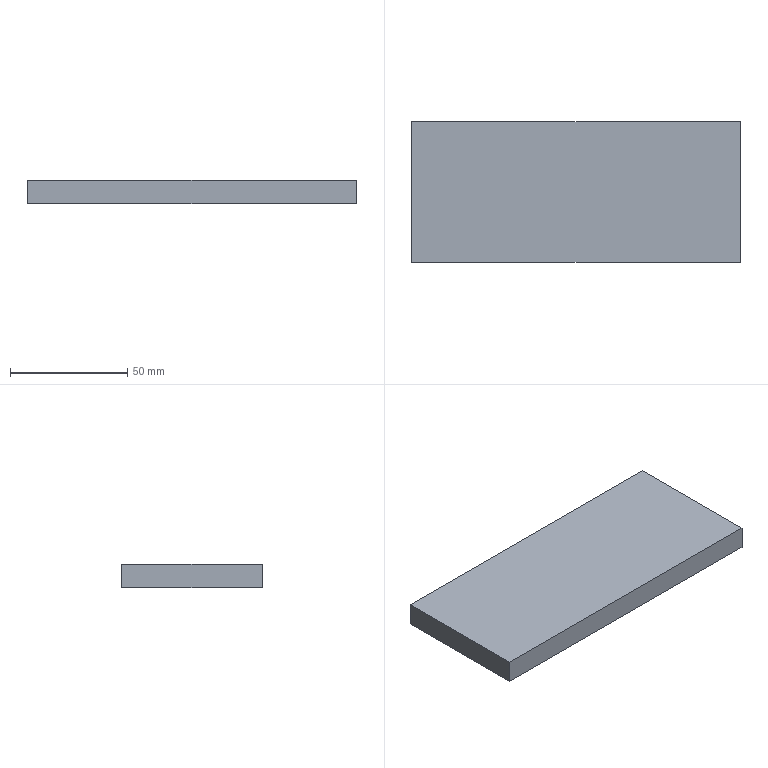Part | SolidWorks | features Extrusion 1 | 1 solid | 6 faces | box 140 x 60 x 10 mm | volume 84000 mm3 | plane 6
STEP:
#1=CARTESIAN_POINT('',(0.,0.,0.));
#2=VERTEX_POINT('',#1);
#3=CARTESIAN_POINT('',(0.,60.,0.));
#4=VERTEX_POINT('',#3);
#5=CARTESIAN_POINT('',(0.,60.,0.));
#6=DIRECTION('',(0.,1.,0.));
#7=VECTOR('',#6,1000.);
#8=LINE('',#5,#7);
#9=EDGE_CURVE('',#2,#4,#8,.T.);
#10=ORIENTED_EDGE('',*,*,#9,.T.);
#11=CARTESIAN_POINT('',(0.,60.,10.));
#12=VERTEX_POINT('',#11);
#13=CARTESIAN_POINT('',(0.,60.,10.));
#14=DIRECTION('',(0.,0.,-1.));
#15=VECTOR('',#14,1000.);
#16=LINE('',#13,#15);
#17=EDGE_CURVE('',#12,#4,#16,.T.);
#18=ORIENTED_EDGE('',*,*,#17,.F.);
#19=CARTESIAN_POINT('',(0.,0.,10.));
#20=VERTEX_POINT('',#19);
#21=CARTESIAN_POINT('',(0.,60.,10.));
#22=DIRECTION('',(0.,1.,0.));
#23=VECTOR('',#22,1000.);
#24=LINE('',#21,#23);
#25=EDGE_CURVE('',#20,#12,#24,.T.);
#26=ORIENTED_EDGE('',*,*,#25,.F.);
#27=CARTESIAN_POINT('',(0.,0.,10.));
#28=DIRECTION('',(0.,0.,-1.));
#29=VECTOR('',#28,1000.);
#30=LINE('',#27,#29);
#31=EDGE_CURVE('',#20,#2,#30,.T.);
#32=ORIENTED_EDGE('',*,*,#31,.T.);
#33=EDGE_LOOP('',(#10,#18,#26,#32));
#34=FACE_OUTER_BOUND('',#33,.T.);
#35=CARTESIAN_POINT('',(0.,60.,10.));
#36=DIRECTION('',(-1.,0.,0.));
#37=DIRECTION('',(0.,0.,1.));
#38=AXIS2_PLACEMENT_3D('',#35,#36,#37);
#39=PLANE('',#38);
#40=ADVANCED_FACE('',(#34),#39,.F.);
#41=CARTESIAN_POINT('',(-140.,60.,0.));
#42=VERTEX_POINT('',#41);
#43=CARTESIAN_POINT('',(-140.,60.,0.));
#44=DIRECTION('',(-1.,0.,0.));
#45=VECTOR('',#44,1000.);
#46=LINE('',#43,#45);
#47=EDGE_CURVE('',#4,#42,#46,.T.);
#48=ORIENTED_EDGE('',*,*,#47,.T.);
#49=CARTESIAN_POINT('',(-140.,60.,10.));
#50=VERTEX_POINT('',#49);
#51=CARTESIAN_POINT('',(-140.,60.,10.));
#52=DIRECTION('',(0.,0.,-1.));
#53=VECTOR('',#52,1000.);
#54=LINE('',#51,#53);
#55=EDGE_CURVE('',#50,#42,#54,.T.);
#56=ORIENTED_EDGE('',*,*,#55,.F.);
#57=CARTESIAN_POINT('',(-140.,60.,10.));
#58=DIRECTION('',(-1.,0.,0.));
#59=VECTOR('',#58,1000.);
#60=LINE('',#57,#59);
#61=EDGE_CURVE('',#12,#50,#60,.T.);
#62=ORIENTED_EDGE('',*,*,#61,.F.);
#63=ORIENTED_EDGE('',*,*,#17,.T.);
#64=EDGE_LOOP('',(#48,#56,#62,#63));
#65=FACE_OUTER_BOUND('',#64,.T.);
#66=CARTESIAN_POINT('',(-140.,60.,10.));
#67=DIRECTION('',(0.,-1.,0.));
#68=DIRECTION('',(0.,0.,-1.));
#69=AXIS2_PLACEMENT_3D('',#66,#67,#68);
#70=PLANE('',#69);
#71=ADVANCED_FACE('',(#65),#70,.F.);
#72=CARTESIAN_POINT('',(-140.,0.,0.));
#73=VERTEX_POINT('',#72);
#74=CARTESIAN_POINT('',(-140.,0.,0.));
#75=DIRECTION('',(0.,-1.,0.));
#76=VECTOR('',#75,1000.);
#77=LINE('',#74,#76);
#78=EDGE_CURVE('',#42,#73,#77,.T.);
#79=ORIENTED_EDGE('',*,*,#78,.T.);
#80=CARTESIAN_POINT('',(-140.,0.,10.));
#81=VERTEX_POINT('',#80);
#82=CARTESIAN_POINT('',(-140.,0.,10.));
#83=DIRECTION('',(0.,0.,-1.));
#84=VECTOR('',#83,1000.);
#85=LINE('',#82,#84);
#86=EDGE_CURVE('',#81,#73,#85,.T.);
#87=ORIENTED_EDGE('',*,*,#86,.F.);
#88=CARTESIAN_POINT('',(-140.,0.,10.));
#89=DIRECTION('',(0.,-1.,0.));
#90=VECTOR('',#89,1000.);
#91=LINE('',#88,#90);
#92=EDGE_CURVE('',#50,#81,#91,.T.);
#93=ORIENTED_EDGE('',*,*,#92,.F.);
#94=ORIENTED_EDGE('',*,*,#55,.T.);
#95=EDGE_LOOP('',(#79,#87,#93,#94));
#96=FACE_OUTER_BOUND('',#95,.T.);
#97=CARTESIAN_POINT('',(-140.,0.,10.));
#98=DIRECTION('',(1.,0.,0.));
#99=DIRECTION('',(0.,0.,-1.));
#100=AXIS2_PLACEMENT_3D('',#97,#98,#99);
#101=PLANE('',#100);
#102=ADVANCED_FACE('',(#96),#101,.F.);
#103=CARTESIAN_POINT('',(0.,0.,0.));
#104=DIRECTION('',(1.,0.,0.));
#105=VECTOR('',#104,1000.);
#106=LINE('',#103,#105);
#107=EDGE_CURVE('',#73,#2,#106,.T.);
#108=ORIENTED_EDGE('',*,*,#107,.T.);
#109=ORIENTED_EDGE('',*,*,#31,.F.);
#110=CARTESIAN_POINT('',(0.,0.,10.));
#111=DIRECTION('',(1.,0.,0.));
#112=VECTOR('',#111,1000.);
#113=LINE('',#110,#112);
#114=EDGE_CURVE('',#81,#20,#113,.T.);
#115=ORIENTED_EDGE('',*,*,#114,.F.);
#116=ORIENTED_EDGE('',*,*,#86,.T.);
#117=EDGE_LOOP('',(#108,#109,#115,#116));
#118=FACE_OUTER_BOUND('',#117,.T.);
#119=CARTESIAN_POINT('',(0.,0.,10.));
#120=DIRECTION('',(0.,1.,0.));
#121=DIRECTION('',(-1.,0.,0.));
#122=AXIS2_PLACEMENT_3D('',#119,#120,#121);
#123=PLANE('',#122);
#124=ADVANCED_FACE('',(#118),#123,.F.);
#125=ORIENTED_EDGE('',*,*,#25,.T.);
#126=ORIENTED_EDGE('',*,*,#61,.T.);
#127=ORIENTED_EDGE('',*,*,#92,.T.);
#128=ORIENTED_EDGE('',*,*,#114,.T.);
#129=EDGE_LOOP('',(#125,#126,#127,#128));
#130=FACE_OUTER_BOUND('',#129,.T.);
#131=CARTESIAN_POINT('',(0.,0.,10.));
#132=DIRECTION('',(0.,0.,-1.));
#133=DIRECTION('',(-1.,0.,0.));
#134=AXIS2_PLACEMENT_3D('',#131,#132,#133);
#135=PLANE('',#134);
#136=ADVANCED_FACE('',(#130),#135,.F.);
#137=ORIENTED_EDGE('',*,*,#9,.F.);
#138=ORIENTED_EDGE('',*,*,#107,.F.);
#139=ORIENTED_EDGE('',*,*,#78,.F.);
#140=ORIENTED_EDGE('',*,*,#47,.F.);
#141=EDGE_LOOP('',(#137,#138,#139,#140));
#142=FACE_OUTER_BOUND('',#141,.T.);
#143=CARTESIAN_POINT('',(0.,0.,0.));
#144=DIRECTION('',(0.,0.,-1.));
#145=DIRECTION('',(-1.,0.,0.));
#146=AXIS2_PLACEMENT_3D('',#143,#144,#145);
#147=PLANE('',#146);
#148=ADVANCED_FACE('',(#142),#147,.T.);
#149=CLOSED_SHELL('',(#40,#71,#102,#124,#136,#148));
#150=MANIFOLD_SOLID_BREP('',#149);
#151=CARTESIAN_POINT('',(0.,0.,0.));
#152=DIRECTION('',(0.,0.,1.));
#153=DIRECTION('',(1.,0.,0.));
#154=AXIS2_PLACEMENT_3D('',#151,#152,#153);
#155=(LENGTH_UNIT()NAMED_UNIT(*)SI_UNIT(.MILLI.,.METRE.));
#156=UNCERTAINTY_MEASURE_WITH_UNIT(LENGTH_MEASURE(0.00001),#155,'','');
#157=(NAMED_UNIT(*)PLANE_ANGLE_UNIT()SI_UNIT($,.RADIAN.));
#158=(NAMED_UNIT(*)SI_UNIT($,.STERADIAN.)SOLID_ANGLE_UNIT());
#159=(GEOMETRIC_REPRESENTATION_CONTEXT(3)GLOBAL_UNCERTAINTY_ASSIGNED_CONTEXT((#156))GLOBAL_UNIT_ASSIGNED_CONTEXT((#155,#157,#158))REPRESENTATION_CONTEXT('',''));
#160=ADVANCED_BREP_SHAPE_REPRESENTATION('',(#150,#154),#159);